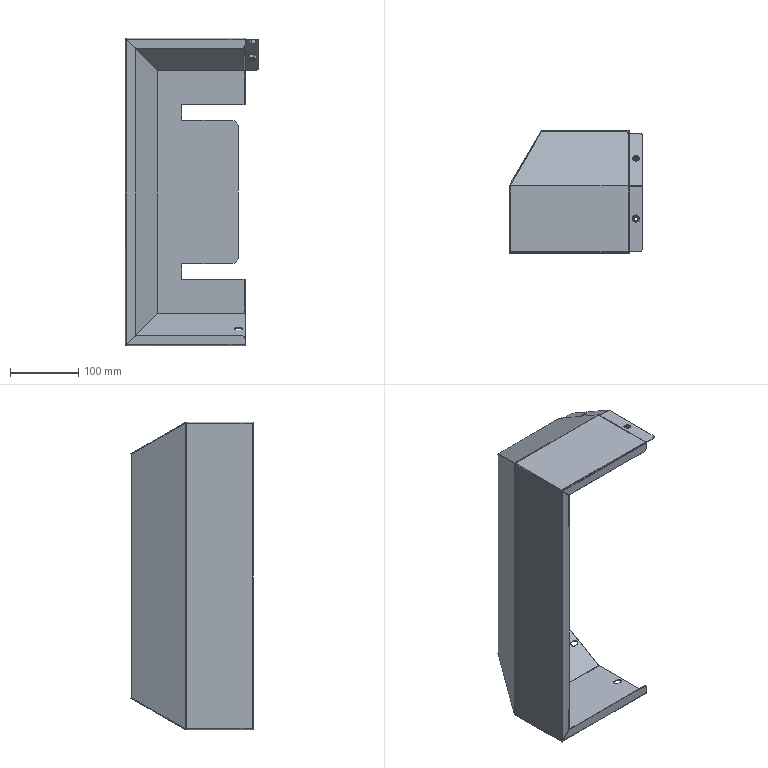Part | STEP file | PN_0018 H244x175 column protective cover_Default<As Machined> | 3 solids | 201 faces | box 195 x 178.808 x 450 mm | volume 198447 mm3 | plane 139 | cylinder 48 | cone 8 | spline 6 | commonest cylinder face diameters 1 x11 3 x11 10 x8 0.4 x4 2.4 x4 7 x4